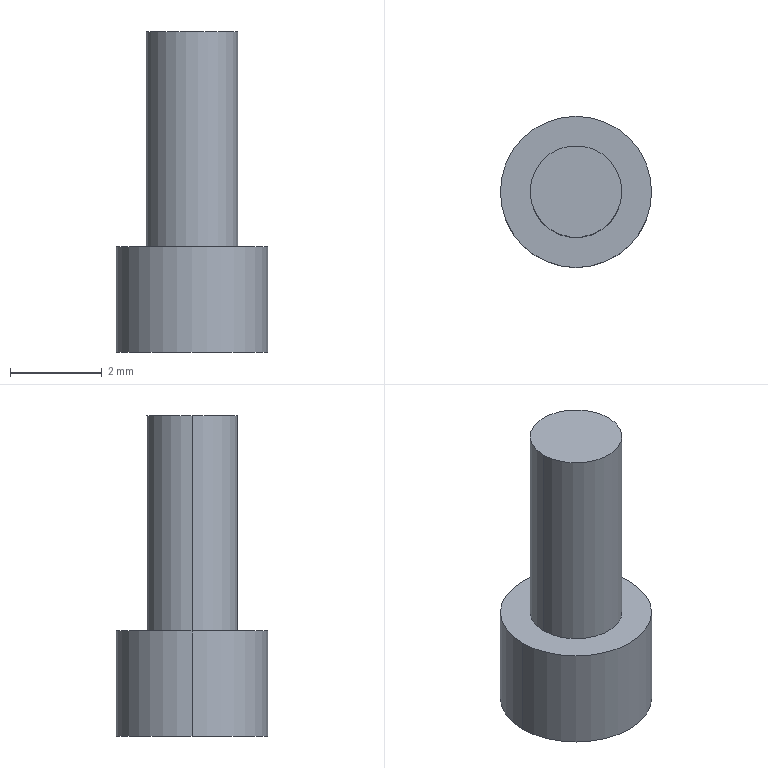Part | SolidWorks | features Extrusion 1, ICE 1 | 1 solid | 7 faces | box 3.3 x 3.3 x 7 mm | volume 34.437 mm3 | cylinder 4 | plane 3 | commonest cylinder face diameters 2 x2 3.3 x2
STEP:
#1=CARTESIAN_POINT('',(1.,0.,7.));
#2=VERTEX_POINT('',#1);
#3=CARTESIAN_POINT('',(-1.,0.,7.));
#4=VERTEX_POINT('',#3);
#5=CARTESIAN_POINT('',(0.,0.,7.));
#6=DIRECTION('',(0.,0.,1.));
#7=DIRECTION('',(1.,0.,0.));
#8=AXIS2_PLACEMENT_3D('',#5,#6,#7);
#9=CIRCLE('',#8,1.);
#10=EDGE_CURVE('',#2,#4,#9,.T.);
#11=ORIENTED_EDGE('',*,*,#10,.F.);
#12=CARTESIAN_POINT('',(1.,0.,2.3));
#13=VERTEX_POINT('',#12);
#14=CARTESIAN_POINT('',(1.,0.,7.));
#15=DIRECTION('',(0.,0.,-1.));
#16=VECTOR('',#15,1000.);
#17=LINE('',#14,#16);
#18=EDGE_CURVE('',#2,#13,#17,.T.);
#19=ORIENTED_EDGE('',*,*,#18,.T.);
#20=CARTESIAN_POINT('',(-1.,0.,2.3));
#21=VERTEX_POINT('',#20);
#22=CARTESIAN_POINT('',(0.,0.,2.3));
#23=DIRECTION('',(0.,0.,1.));
#24=DIRECTION('',(1.,0.,0.));
#25=AXIS2_PLACEMENT_3D('',#22,#23,#24);
#26=CIRCLE('',#25,1.);
#27=EDGE_CURVE('',#13,#21,#26,.T.);
#28=ORIENTED_EDGE('',*,*,#27,.T.);
#29=CARTESIAN_POINT('',(-1.,0.,7.));
#30=DIRECTION('',(0.,0.,-1.));
#31=VECTOR('',#30,1000.);
#32=LINE('',#29,#31);
#33=EDGE_CURVE('',#4,#21,#32,.T.);
#34=ORIENTED_EDGE('',*,*,#33,.F.);
#35=EDGE_LOOP('',(#11,#19,#28,#34));
#36=FACE_OUTER_BOUND('',#35,.T.);
#37=CARTESIAN_POINT('',(0.,0.,7.));
#38=DIRECTION('',(0.,0.,-1.));
#39=DIRECTION('',(-1.,0.,0.));
#40=AXIS2_PLACEMENT_3D('',#37,#38,#39);
#41=CYLINDRICAL_SURFACE('',#40,1.);
#42=ADVANCED_FACE('',(#36),#41,.T.);
#43=CARTESIAN_POINT('',(1.65,0.,2.3));
#44=VERTEX_POINT('',#43);
#45=CARTESIAN_POINT('',(-1.65,0.,2.3));
#46=VERTEX_POINT('',#45);
#47=CARTESIAN_POINT('',(0.,0.,2.3));
#48=DIRECTION('',(0.,0.,1.));
#49=DIRECTION('',(1.,0.,0.));
#50=AXIS2_PLACEMENT_3D('',#47,#48,#49);
#51=CIRCLE('',#50,1.65);
#52=EDGE_CURVE('',#44,#46,#51,.T.);
#53=ORIENTED_EDGE('',*,*,#52,.F.);
#54=CARTESIAN_POINT('',(1.65,0.,0.));
#55=VERTEX_POINT('',#54);
#56=CARTESIAN_POINT('',(1.65,0.,2.3));
#57=DIRECTION('',(0.,0.,-1.));
#58=VECTOR('',#57,1000.);
#59=LINE('',#56,#58);
#60=EDGE_CURVE('',#44,#55,#59,.T.);
#61=ORIENTED_EDGE('',*,*,#60,.T.);
#62=CARTESIAN_POINT('',(-1.65,0.,0.));
#63=VERTEX_POINT('',#62);
#64=CARTESIAN_POINT('',(0.,0.,0.));
#65=DIRECTION('',(0.,0.,1.));
#66=DIRECTION('',(1.,0.,0.));
#67=AXIS2_PLACEMENT_3D('',#64,#65,#66);
#68=CIRCLE('',#67,1.65);
#69=EDGE_CURVE('',#55,#63,#68,.T.);
#70=ORIENTED_EDGE('',*,*,#69,.T.);
#71=CARTESIAN_POINT('',(-1.65,0.,2.3));
#72=DIRECTION('',(0.,0.,-1.));
#73=VECTOR('',#72,1000.);
#74=LINE('',#71,#73);
#75=EDGE_CURVE('',#46,#63,#74,.T.);
#76=ORIENTED_EDGE('',*,*,#75,.F.);
#77=EDGE_LOOP('',(#53,#61,#70,#76));
#78=FACE_OUTER_BOUND('',#77,.T.);
#79=CARTESIAN_POINT('',(0.,0.,2.3));
#80=DIRECTION('',(0.,0.,-1.));
#81=DIRECTION('',(-1.,0.,0.));
#82=AXIS2_PLACEMENT_3D('',#79,#80,#81);
#83=CYLINDRICAL_SURFACE('',#82,1.65);
#84=ADVANCED_FACE('',(#78),#83,.T.);
#85=ORIENTED_EDGE('',*,*,#60,.F.);
#86=CARTESIAN_POINT('',(0.,0.,2.3));
#87=DIRECTION('',(0.,0.,1.));
#88=DIRECTION('',(1.,0.,0.));
#89=AXIS2_PLACEMENT_3D('',#86,#87,#88);
#90=CIRCLE('',#89,1.65);
#91=EDGE_CURVE('',#46,#44,#90,.T.);
#92=ORIENTED_EDGE('',*,*,#91,.F.);
#93=ORIENTED_EDGE('',*,*,#75,.T.);
#94=CARTESIAN_POINT('',(0.,0.,0.));
#95=DIRECTION('',(0.,0.,1.));
#96=DIRECTION('',(1.,0.,0.));
#97=AXIS2_PLACEMENT_3D('',#94,#95,#96);
#98=CIRCLE('',#97,1.65);
#99=EDGE_CURVE('',#63,#55,#98,.T.);
#100=ORIENTED_EDGE('',*,*,#99,.T.);
#101=EDGE_LOOP('',(#85,#92,#93,#100));
#102=FACE_OUTER_BOUND('',#101,.T.);
#103=CARTESIAN_POINT('',(0.,0.,2.3));
#104=DIRECTION('',(0.,0.,-1.));
#105=DIRECTION('',(-1.,0.,0.));
#106=AXIS2_PLACEMENT_3D('',#103,#104,#105);
#107=CYLINDRICAL_SURFACE('',#106,1.65);
#108=ADVANCED_FACE('',(#102),#107,.T.);
#109=CARTESIAN_POINT('',(0.,0.,2.3));
#110=DIRECTION('',(0.,0.,1.));
#111=DIRECTION('',(1.,0.,0.));
#112=AXIS2_PLACEMENT_3D('',#109,#110,#111);
#113=CIRCLE('',#112,1.);
#114=EDGE_CURVE('',#21,#13,#113,.T.);
#115=ORIENTED_EDGE('',*,*,#114,.F.);
#116=ORIENTED_EDGE('',*,*,#27,.F.);
#117=EDGE_LOOP('',(#115,#116));
#118=FACE_BOUND('',#117,.T.);
#119=ORIENTED_EDGE('',*,*,#91,.T.);
#120=ORIENTED_EDGE('',*,*,#52,.T.);
#121=EDGE_LOOP('',(#119,#120));
#122=FACE_OUTER_BOUND('',#121,.T.);
#123=CARTESIAN_POINT('',(0.,0.,2.3));
#124=DIRECTION('',(0.,0.,1.));
#125=DIRECTION('',(1.,0.,0.));
#126=AXIS2_PLACEMENT_3D('',#123,#124,#125);
#127=PLANE('',#126);
#128=ADVANCED_FACE('',(#118,#122),#127,.T.);
#129=ORIENTED_EDGE('',*,*,#99,.F.);
#130=ORIENTED_EDGE('',*,*,#69,.F.);
#131=EDGE_LOOP('',(#129,#130));
#132=FACE_OUTER_BOUND('',#131,.T.);
#133=CARTESIAN_POINT('',(0.,0.,0.));
#134=DIRECTION('',(0.,0.,1.));
#135=DIRECTION('',(1.,0.,0.));
#136=AXIS2_PLACEMENT_3D('',#133,#134,#135);
#137=PLANE('',#136);
#138=ADVANCED_FACE('',(#132),#137,.F.);
#139=ORIENTED_EDGE('',*,*,#18,.F.);
#140=CARTESIAN_POINT('',(0.,0.,7.));
#141=DIRECTION('',(0.,0.,1.));
#142=DIRECTION('',(1.,0.,0.));
#143=AXIS2_PLACEMENT_3D('',#140,#141,#142);
#144=CIRCLE('',#143,1.);
#145=EDGE_CURVE('',#4,#2,#144,.T.);
#146=ORIENTED_EDGE('',*,*,#145,.F.);
#147=ORIENTED_EDGE('',*,*,#33,.T.);
#148=ORIENTED_EDGE('',*,*,#114,.T.);
#149=EDGE_LOOP('',(#139,#146,#147,#148));
#150=FACE_OUTER_BOUND('',#149,.T.);
#151=CARTESIAN_POINT('',(0.,0.,7.));
#152=DIRECTION('',(0.,0.,-1.));
#153=DIRECTION('',(-1.,0.,0.));
#154=AXIS2_PLACEMENT_3D('',#151,#152,#153);
#155=CYLINDRICAL_SURFACE('',#154,1.);
#156=ADVANCED_FACE('',(#150),#155,.T.);
#157=ORIENTED_EDGE('',*,*,#145,.T.);
#158=ORIENTED_EDGE('',*,*,#10,.T.);
#159=EDGE_LOOP('',(#157,#158));
#160=FACE_OUTER_BOUND('',#159,.T.);
#161=CARTESIAN_POINT('',(0.,0.,7.));
#162=DIRECTION('',(0.,0.,1.));
#163=DIRECTION('',(1.,0.,0.));
#164=AXIS2_PLACEMENT_3D('',#161,#162,#163);
#165=PLANE('',#164);
#166=ADVANCED_FACE('',(#160),#165,.T.);
#167=CLOSED_SHELL('',(#42,#84,#108,#128,#138,#156,#166));
#168=MANIFOLD_SOLID_BREP('',#167);
#169=CARTESIAN_POINT('',(0.,0.,0.));
#170=DIRECTION('',(0.,0.,1.));
#171=DIRECTION('',(1.,0.,0.));
#172=AXIS2_PLACEMENT_3D('',#169,#170,#171);
#173=(LENGTH_UNIT()NAMED_UNIT(*)SI_UNIT(.MILLI.,.METRE.));
#174=UNCERTAINTY_MEASURE_WITH_UNIT(LENGTH_MEASURE(0.00001),#173,'','');
#175=(NAMED_UNIT(*)PLANE_ANGLE_UNIT()SI_UNIT($,.RADIAN.));
#176=(NAMED_UNIT(*)SI_UNIT($,.STERADIAN.)SOLID_ANGLE_UNIT());
#177=(GEOMETRIC_REPRESENTATION_CONTEXT(3)GLOBAL_UNCERTAINTY_ASSIGNED_CONTEXT((#174))GLOBAL_UNIT_ASSIGNED_CONTEXT((#173,#175,#176))REPRESENTATION_CONTEXT('',''));
#178=ADVANCED_BREP_SHAPE_REPRESENTATION('',(#168,#172),#177);